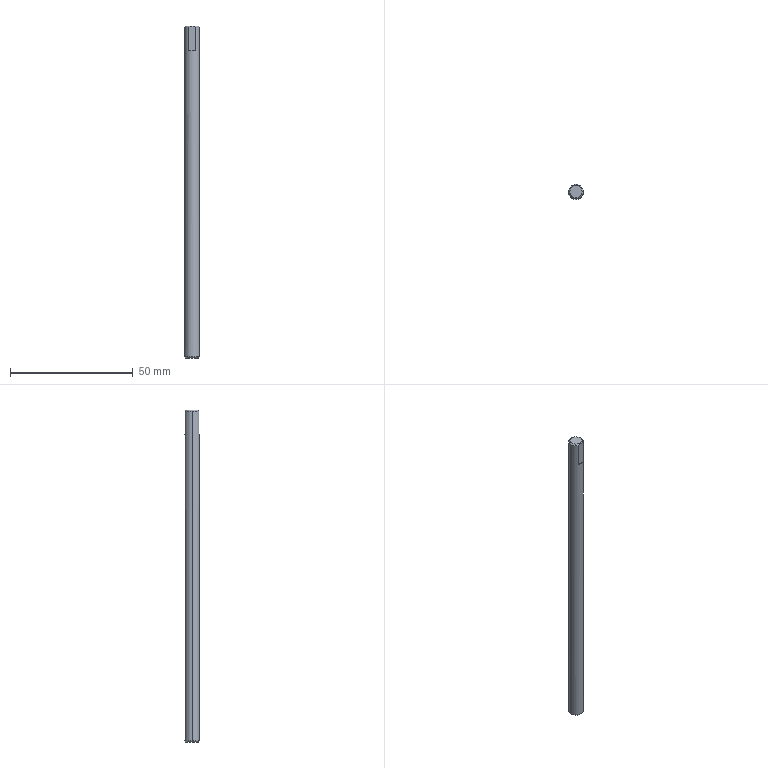Part | STEP file | 11-FG-B05111 | 1 solid | 12 faces | box 6 x 6 x 135 mm | volume 3802 mm3 | plane 6 | cone 4 | cylinder 2 | commonest cylinder face diameters 6 x2
STEP:
#1=CARTESIAN_POINT('',(-2.5,0.,0.));
#2=VERTEX_POINT('',#1);
#3=CARTESIAN_POINT('',(2.5,0.,0.));
#4=VERTEX_POINT('',#3);
#5=CARTESIAN_POINT('',(0.,0.,0.));
#6=DIRECTION('',(0.,0.,-1.));
#7=DIRECTION('',(1.,0.,0.));
#8=AXIS2_PLACEMENT_3D('',#5,#6,#7);
#9=CIRCLE('',#8,2.5);
#10=EDGE_CURVE('',#2,#4,#9,.T.);
#11=ORIENTED_EDGE('',*,*,#10,.F.);
#12=CARTESIAN_POINT('',(-3.,0.,0.5));
#13=VERTEX_POINT('',#12);
#14=CARTESIAN_POINT('',(-3.,0.,0.5));
#15=DIRECTION('',(-0.7071,0.,0.7071));
#16=VECTOR('',#15,1000.);
#17=LINE('',#14,#16);
#18=EDGE_CURVE('',#2,#13,#17,.T.);
#19=ORIENTED_EDGE('',*,*,#18,.T.);
#20=CARTESIAN_POINT('',(3.,0.,0.5));
#21=VERTEX_POINT('',#20);
#22=CARTESIAN_POINT('',(0.,0.,0.5));
#23=DIRECTION('',(0.,0.,1.));
#24=DIRECTION('',(1.,0.,0.));
#25=AXIS2_PLACEMENT_3D('',#22,#23,#24);
#26=CIRCLE('',#25,3.);
#27=EDGE_CURVE('',#21,#13,#26,.T.);
#28=ORIENTED_EDGE('',*,*,#27,.F.);
#29=CARTESIAN_POINT('',(3.,0.,0.5));
#30=DIRECTION('',(0.7071,0.,0.7071));
#31=VECTOR('',#30,1000.);
#32=LINE('',#29,#31);
#33=EDGE_CURVE('',#4,#21,#32,.T.);
#34=ORIENTED_EDGE('',*,*,#33,.F.);
#35=EDGE_LOOP('',(#11,#19,#28,#34));
#36=FACE_OUTER_BOUND('',#35,.T.);
#37=CARTESIAN_POINT('',(0.,0.,0.5));
#38=DIRECTION('',(0.,0.,1.));
#39=DIRECTION('',(1.,0.,0.));
#40=AXIS2_PLACEMENT_3D('',#37,#38,#39);
#41=CONICAL_SURFACE('',#40,3.,0.7854);
#42=ADVANCED_FACE('',(#36),#41,.T.);
#43=CARTESIAN_POINT('',(2.5,0.,135.));
#44=VERTEX_POINT('',#43);
#45=CARTESIAN_POINT('',(-2.5,0.,135.));
#46=VERTEX_POINT('',#45);
#47=CARTESIAN_POINT('',(0.,0.,135.));
#48=DIRECTION('',(0.,0.,1.));
#49=DIRECTION('',(1.,0.,0.));
#50=AXIS2_PLACEMENT_3D('',#47,#48,#49);
#51=CIRCLE('',#50,2.5);
#52=EDGE_CURVE('',#44,#46,#51,.T.);
#53=ORIENTED_EDGE('',*,*,#52,.F.);
#54=CARTESIAN_POINT('',(3.,0.,134.5));
#55=VERTEX_POINT('',#54);
#56=CARTESIAN_POINT('',(2.5,0.,135.));
#57=DIRECTION('',(0.7071,0.,-0.7071));
#58=VECTOR('',#57,1000.);
#59=LINE('',#56,#58);
#60=EDGE_CURVE('',#44,#55,#59,.T.);
#61=ORIENTED_EDGE('',*,*,#60,.T.);
#62=CARTESIAN_POINT('',(1.308,2.7,134.5));
#63=VERTEX_POINT('',#62);
#64=CARTESIAN_POINT('',(0.,0.,134.5));
#65=DIRECTION('',(0.,0.,-1.));
#66=DIRECTION('',(1.,0.,0.));
#67=AXIS2_PLACEMENT_3D('',#64,#65,#66);
#68=CIRCLE('',#67,3.);
#69=EDGE_CURVE('',#63,#55,#68,.T.);
#70=ORIENTED_EDGE('',*,*,#69,.F.);
#71=CARTESIAN_POINT('',(-1.308,2.7,134.5));
#72=VERTEX_POINT('',#71);
#73=CARTESIAN_POINT('',(-1.308,2.7,134.5));
#74=CARTESIAN_POINT('',(-1.102,2.7,134.59));
#75=CARTESIAN_POINT('',(-0.8871,2.7,134.666));
#76=CARTESIAN_POINT('',(-0.4489,2.7,134.771));
#77=CARTESIAN_POINT('',(-0.223,2.7,134.8));
#78=CARTESIAN_POINT('',(0.2287,2.7,134.8));
#79=CARTESIAN_POINT('',(0.4505,2.7,134.771));
#80=CARTESIAN_POINT('',(0.8872,2.7,134.666));
#81=CARTESIAN_POINT('',(1.102,2.7,134.59));
#82=CARTESIAN_POINT('',(1.308,2.7,134.5));
#83=B_SPLINE_CURVE_WITH_KNOTS('',3,(#73,#74,#75,#76,#77,#78,#79,#80,#81,#82),.UNSPECIFIED.,.F.,.F.,(4,2,2,2,4),(0.001666,0.002335,0.003005,0.003674,0.004344),.UNSPECIFIED.);
#84=EDGE_CURVE('',#72,#63,#83,.T.);
#85=ORIENTED_EDGE('',*,*,#84,.F.);
#86=CARTESIAN_POINT('',(-3.,0.,134.5));
#87=VERTEX_POINT('',#86);
#88=CARTESIAN_POINT('',(0.,0.,134.5));
#89=DIRECTION('',(0.,0.,-1.));
#90=DIRECTION('',(1.,0.,0.));
#91=AXIS2_PLACEMENT_3D('',#88,#89,#90);
#92=CIRCLE('',#91,3.);
#93=EDGE_CURVE('',#87,#72,#92,.T.);
#94=ORIENTED_EDGE('',*,*,#93,.F.);
#95=CARTESIAN_POINT('',(-2.5,0.,135.));
#96=DIRECTION('',(-0.7071,0.,-0.7071));
#97=VECTOR('',#96,1000.);
#98=LINE('',#95,#97);
#99=EDGE_CURVE('',#46,#87,#98,.T.);
#100=ORIENTED_EDGE('',*,*,#99,.F.);
#101=EDGE_LOOP('',(#53,#61,#70,#85,#94,#100));
#102=FACE_OUTER_BOUND('',#101,.T.);
#103=CARTESIAN_POINT('',(0.,0.,135.));
#104=DIRECTION('',(0.,0.,-1.));
#105=DIRECTION('',(-1.,0.,0.));
#106=AXIS2_PLACEMENT_3D('',#103,#104,#105);
#107=CONICAL_SURFACE('',#106,2.5,0.7854);
#108=ADVANCED_FACE('',(#102),#107,.T.);
#109=ORIENTED_EDGE('',*,*,#69,.T.);
#110=CARTESIAN_POINT('',(3.,0.,135.));
#111=DIRECTION('',(0.,0.,-1.));
#112=VECTOR('',#111,1000.);
#113=LINE('',#110,#112);
#114=EDGE_CURVE('',#55,#21,#113,.T.);
#115=ORIENTED_EDGE('',*,*,#114,.T.);
#116=ORIENTED_EDGE('',*,*,#27,.T.);
#117=CARTESIAN_POINT('',(-3.,0.,135.));
#118=DIRECTION('',(0.,0.,-1.));
#119=VECTOR('',#118,1000.);
#120=LINE('',#117,#119);
#121=EDGE_CURVE('',#87,#13,#120,.T.);
#122=ORIENTED_EDGE('',*,*,#121,.F.);
#123=ORIENTED_EDGE('',*,*,#93,.T.);
#124=CARTESIAN_POINT('',(-1.308,2.7,125.));
#125=VERTEX_POINT('',#124);
#126=CARTESIAN_POINT('',(-1.308,2.7,125.));
#127=DIRECTION('',(0.,0.,1.));
#128=VECTOR('',#127,1000.);
#129=LINE('',#126,#128);
#130=EDGE_CURVE('',#125,#72,#129,.T.);
#131=ORIENTED_EDGE('',*,*,#130,.F.);
#132=CARTESIAN_POINT('',(1.308,2.7,125.));
#133=VERTEX_POINT('',#132);
#134=CARTESIAN_POINT('',(0.,0.,125.));
#135=DIRECTION('',(0.,0.,1.));
#136=DIRECTION('',(1.,0.,0.));
#137=AXIS2_PLACEMENT_3D('',#134,#135,#136);
#138=CIRCLE('',#137,3.);
#139=EDGE_CURVE('',#133,#125,#138,.T.);
#140=ORIENTED_EDGE('',*,*,#139,.F.);
#141=CARTESIAN_POINT('',(1.308,2.7,125.));
#142=DIRECTION('',(0.,0.,1.));
#143=VECTOR('',#142,1000.);
#144=LINE('',#141,#143);
#145=EDGE_CURVE('',#133,#63,#144,.T.);
#146=ORIENTED_EDGE('',*,*,#145,.T.);
#147=EDGE_LOOP('',(#109,#115,#116,#122,#123,#131,#140,#146));
#148=FACE_OUTER_BOUND('',#147,.T.);
#149=CARTESIAN_POINT('',(0.,0.,135.));
#150=DIRECTION('',(0.,0.,-1.));
#151=DIRECTION('',(-1.,0.,0.));
#152=AXIS2_PLACEMENT_3D('',#149,#150,#151);
#153=CYLINDRICAL_SURFACE('',#152,3.);
#154=ADVANCED_FACE('',(#148),#153,.T.);
#155=ORIENTED_EDGE('',*,*,#114,.F.);
#156=CARTESIAN_POINT('',(1.308,-2.7,134.5));
#157=VERTEX_POINT('',#156);
#158=CARTESIAN_POINT('',(0.,0.,134.5));
#159=DIRECTION('',(0.,0.,-1.));
#160=DIRECTION('',(1.,0.,0.));
#161=AXIS2_PLACEMENT_3D('',#158,#159,#160);
#162=CIRCLE('',#161,3.);
#163=EDGE_CURVE('',#55,#157,#162,.T.);
#164=ORIENTED_EDGE('',*,*,#163,.T.);
#165=CARTESIAN_POINT('',(1.308,-2.7,125.));
#166=VERTEX_POINT('',#165);
#167=CARTESIAN_POINT('',(1.308,-2.7,125.));
#168=DIRECTION('',(0.,0.,1.));
#169=VECTOR('',#168,1000.);
#170=LINE('',#167,#169);
#171=EDGE_CURVE('',#166,#157,#170,.T.);
#172=ORIENTED_EDGE('',*,*,#171,.F.);
#173=CARTESIAN_POINT('',(-1.308,-2.7,125.));
#174=VERTEX_POINT('',#173);
#175=CARTESIAN_POINT('',(0.,0.,125.));
#176=DIRECTION('',(0.,0.,1.));
#177=DIRECTION('',(1.,0.,0.));
#178=AXIS2_PLACEMENT_3D('',#175,#176,#177);
#179=CIRCLE('',#178,3.);
#180=EDGE_CURVE('',#174,#166,#179,.T.);
#181=ORIENTED_EDGE('',*,*,#180,.F.);
#182=CARTESIAN_POINT('',(-1.308,-2.7,134.5));
#183=VERTEX_POINT('',#182);
#184=CARTESIAN_POINT('',(-1.308,-2.7,125.));
#185=DIRECTION('',(0.,0.,1.));
#186=VECTOR('',#185,1000.);
#187=LINE('',#184,#186);
#188=EDGE_CURVE('',#174,#183,#187,.T.);
#189=ORIENTED_EDGE('',*,*,#188,.T.);
#190=CARTESIAN_POINT('',(0.,0.,134.5));
#191=DIRECTION('',(0.,0.,-1.));
#192=DIRECTION('',(1.,0.,0.));
#193=AXIS2_PLACEMENT_3D('',#190,#191,#192);
#194=CIRCLE('',#193,3.);
#195=EDGE_CURVE('',#183,#87,#194,.T.);
#196=ORIENTED_EDGE('',*,*,#195,.T.);
#197=ORIENTED_EDGE('',*,*,#121,.T.);
#198=CARTESIAN_POINT('',(0.,0.,0.5));
#199=DIRECTION('',(0.,0.,1.));
#200=DIRECTION('',(1.,0.,0.));
#201=AXIS2_PLACEMENT_3D('',#198,#199,#200);
#202=CIRCLE('',#201,3.);
#203=EDGE_CURVE('',#13,#21,#202,.T.);
#204=ORIENTED_EDGE('',*,*,#203,.T.);
#205=EDGE_LOOP('',(#155,#164,#172,#181,#189,#196,#197,#204));
#206=FACE_OUTER_BOUND('',#205,.T.);
#207=CARTESIAN_POINT('',(0.,0.,135.));
#208=DIRECTION('',(0.,0.,-1.));
#209=DIRECTION('',(-1.,0.,0.));
#210=AXIS2_PLACEMENT_3D('',#207,#208,#209);
#211=CYLINDRICAL_SURFACE('',#210,3.);
#212=ADVANCED_FACE('',(#206),#211,.T.);
#213=CARTESIAN_POINT('',(0.,0.,135.));
#214=DIRECTION('',(0.,0.,1.));
#215=DIRECTION('',(1.,0.,0.));
#216=AXIS2_PLACEMENT_3D('',#213,#214,#215);
#217=CIRCLE('',#216,2.5);
#218=EDGE_CURVE('',#46,#44,#217,.T.);
#219=ORIENTED_EDGE('',*,*,#218,.T.);
#220=ORIENTED_EDGE('',*,*,#52,.T.);
#221=EDGE_LOOP('',(#219,#220));
#222=FACE_OUTER_BOUND('',#221,.T.);
#223=CARTESIAN_POINT('',(0.,0.,135.));
#224=DIRECTION('',(0.,0.,1.));
#225=DIRECTION('',(1.,0.,0.));
#226=AXIS2_PLACEMENT_3D('',#223,#224,#225);
#227=PLANE('',#226);
#228=ADVANCED_FACE('',(#222),#227,.T.);
#229=CARTESIAN_POINT('',(0.,0.,0.));
#230=DIRECTION('',(0.,0.,-1.));
#231=DIRECTION('',(1.,0.,0.));
#232=AXIS2_PLACEMENT_3D('',#229,#230,#231);
#233=CIRCLE('',#232,2.5);
#234=EDGE_CURVE('',#4,#2,#233,.T.);
#235=ORIENTED_EDGE('',*,*,#234,.T.);
#236=ORIENTED_EDGE('',*,*,#10,.T.);
#237=EDGE_LOOP('',(#235,#236));
#238=FACE_OUTER_BOUND('',#237,.T.);
#239=CARTESIAN_POINT('',(0.,0.,0.));
#240=DIRECTION('',(0.,0.,1.));
#241=DIRECTION('',(1.,0.,0.));
#242=AXIS2_PLACEMENT_3D('',#239,#240,#241);
#243=PLANE('',#242);
#244=ADVANCED_FACE('',(#238),#243,.F.);
#245=ORIENTED_EDGE('',*,*,#60,.F.);
#246=ORIENTED_EDGE('',*,*,#218,.F.);
#247=ORIENTED_EDGE('',*,*,#99,.T.);
#248=ORIENTED_EDGE('',*,*,#195,.F.);
#249=CARTESIAN_POINT('',(1.308,-2.7,134.5));
#250=CARTESIAN_POINT('',(1.102,-2.7,134.59));
#251=CARTESIAN_POINT('',(0.8872,-2.7,134.666));
#252=CARTESIAN_POINT('',(0.4505,-2.7,134.771));
#253=CARTESIAN_POINT('',(0.2287,-2.7,134.8));
#254=CARTESIAN_POINT('',(-0.223,-2.7,134.8));
#255=CARTESIAN_POINT('',(-0.4489,-2.7,134.771));
#256=CARTESIAN_POINT('',(-0.8871,-2.7,134.666));
#257=CARTESIAN_POINT('',(-1.102,-2.7,134.59));
#258=CARTESIAN_POINT('',(-1.308,-2.7,134.5));
#259=B_SPLINE_CURVE_WITH_KNOTS('',3,(#249,#250,#251,#252,#253,#254,#255,#256,#257,#258),.UNSPECIFIED.,.F.,.F.,(4,2,2,2,4),(0.001237,0.001908,0.002579,0.00325,0.003921),.UNSPECIFIED.);
#260=EDGE_CURVE('',#157,#183,#259,.T.);
#261=ORIENTED_EDGE('',*,*,#260,.F.);
#262=ORIENTED_EDGE('',*,*,#163,.F.);
#263=EDGE_LOOP('',(#245,#246,#247,#248,#261,#262));
#264=FACE_OUTER_BOUND('',#263,.T.);
#265=CARTESIAN_POINT('',(0.,0.,135.));
#266=DIRECTION('',(0.,0.,-1.));
#267=DIRECTION('',(-1.,0.,0.));
#268=AXIS2_PLACEMENT_3D('',#265,#266,#267);
#269=CONICAL_SURFACE('',#268,2.5,0.7854);
#270=ADVANCED_FACE('',(#264),#269,.T.);
#271=ORIENTED_EDGE('',*,*,#18,.F.);
#272=ORIENTED_EDGE('',*,*,#234,.F.);
#273=ORIENTED_EDGE('',*,*,#33,.T.);
#274=ORIENTED_EDGE('',*,*,#203,.F.);
#275=EDGE_LOOP('',(#271,#272,#273,#274));
#276=FACE_OUTER_BOUND('',#275,.T.);
#277=CARTESIAN_POINT('',(0.,0.,0.5));
#278=DIRECTION('',(0.,0.,1.));
#279=DIRECTION('',(1.,0.,0.));
#280=AXIS2_PLACEMENT_3D('',#277,#278,#279);
#281=CONICAL_SURFACE('',#280,3.,0.7854);
#282=ADVANCED_FACE('',(#276),#281,.T.);
#283=ORIENTED_EDGE('',*,*,#84,.T.);
#284=ORIENTED_EDGE('',*,*,#145,.F.);
#285=CARTESIAN_POINT('',(-1.308,2.7,125.));
#286=DIRECTION('',(1.,0.,0.));
#287=VECTOR('',#286,1000.);
#288=LINE('',#285,#287);
#289=EDGE_CURVE('',#125,#133,#288,.T.);
#290=ORIENTED_EDGE('',*,*,#289,.F.);
#291=ORIENTED_EDGE('',*,*,#130,.T.);
#292=EDGE_LOOP('',(#283,#284,#290,#291));
#293=FACE_OUTER_BOUND('',#292,.T.);
#294=CARTESIAN_POINT('',(-1.308,2.7,125.));
#295=DIRECTION('',(0.,-1.,0.));
#296=DIRECTION('',(1.,0.,0.));
#297=AXIS2_PLACEMENT_3D('',#294,#295,#296);
#298=PLANE('',#297);
#299=ADVANCED_FACE('',(#293),#298,.F.);
#300=ORIENTED_EDGE('',*,*,#139,.T.);
#301=ORIENTED_EDGE('',*,*,#289,.T.);
#302=EDGE_LOOP('',(#300,#301));
#303=FACE_OUTER_BOUND('',#302,.T.);
#304=CARTESIAN_POINT('',(0.,0.,125.));
#305=DIRECTION('',(0.,0.,1.));
#306=DIRECTION('',(1.,0.,0.));
#307=AXIS2_PLACEMENT_3D('',#304,#305,#306);
#308=PLANE('',#307);
#309=ADVANCED_FACE('',(#303),#308,.T.);
#310=ORIENTED_EDGE('',*,*,#260,.T.);
#311=ORIENTED_EDGE('',*,*,#188,.F.);
#312=CARTESIAN_POINT('',(-1.308,-2.7,125.));
#313=DIRECTION('',(-1.,0.,0.));
#314=VECTOR('',#313,1000.);
#315=LINE('',#312,#314);
#316=EDGE_CURVE('',#166,#174,#315,.T.);
#317=ORIENTED_EDGE('',*,*,#316,.F.);
#318=ORIENTED_EDGE('',*,*,#171,.T.);
#319=EDGE_LOOP('',(#310,#311,#317,#318));
#320=FACE_OUTER_BOUND('',#319,.T.);
#321=CARTESIAN_POINT('',(-1.308,-2.7,125.));
#322=DIRECTION('',(0.,1.,0.));
#323=DIRECTION('',(-1.,0.,0.));
#324=AXIS2_PLACEMENT_3D('',#321,#322,#323);
#325=PLANE('',#324);
#326=ADVANCED_FACE('',(#320),#325,.F.);
#327=ORIENTED_EDGE('',*,*,#180,.T.);
#328=ORIENTED_EDGE('',*,*,#316,.T.);
#329=EDGE_LOOP('',(#327,#328));
#330=FACE_OUTER_BOUND('',#329,.T.);
#331=CARTESIAN_POINT('',(0.,0.,125.));
#332=DIRECTION('',(0.,0.,1.));
#333=DIRECTION('',(1.,0.,0.));
#334=AXIS2_PLACEMENT_3D('',#331,#332,#333);
#335=PLANE('',#334);
#336=ADVANCED_FACE('',(#330),#335,.T.);
#337=CLOSED_SHELL('',(#42,#108,#154,#212,#228,#244,#270,#282,#299,#309,#326,#336));
#338=MANIFOLD_SOLID_BREP('',#337);
#339=CARTESIAN_POINT('',(0.,0.,0.));
#340=DIRECTION('',(0.,0.,1.));
#341=DIRECTION('',(1.,0.,0.));
#342=AXIS2_PLACEMENT_3D('',#339,#340,#341);
#343=(LENGTH_UNIT()NAMED_UNIT(*)SI_UNIT(.MILLI.,.METRE.));
#344=UNCERTAINTY_MEASURE_WITH_UNIT(LENGTH_MEASURE(0.00001),#343,'','');
#345=(NAMED_UNIT(*)PLANE_ANGLE_UNIT()SI_UNIT($,.RADIAN.));
#346=(NAMED_UNIT(*)SI_UNIT($,.STERADIAN.)SOLID_ANGLE_UNIT());
#347=(GEOMETRIC_REPRESENTATION_CONTEXT(3)GLOBAL_UNCERTAINTY_ASSIGNED_CONTEXT((#344))GLOBAL_UNIT_ASSIGNED_CONTEXT((#343,#345,#346))REPRESENTATION_CONTEXT('',''));
#348=ADVANCED_BREP_SHAPE_REPRESENTATION('',(#338,#342),#347);